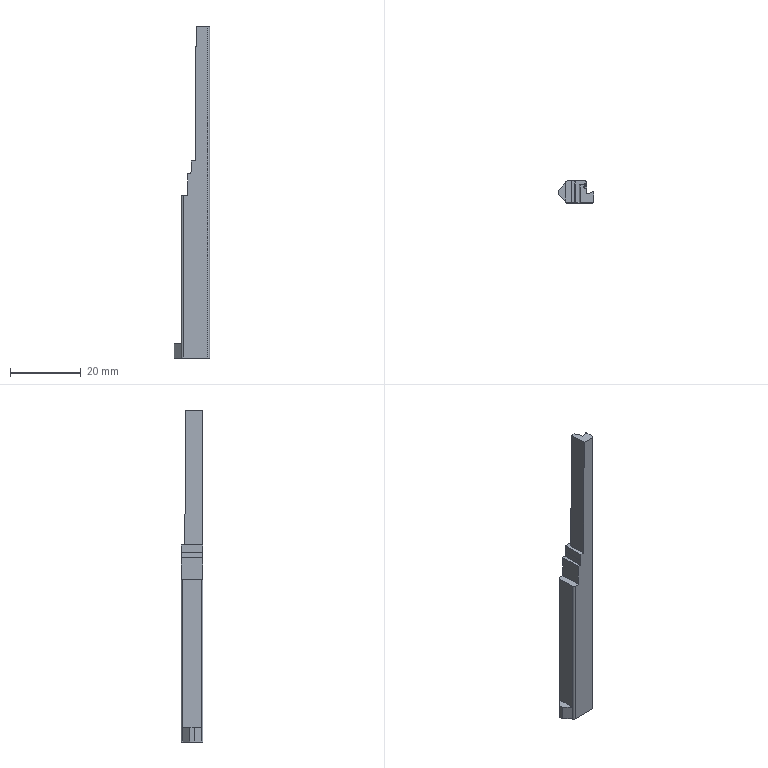Part | Creo | 1 solid | 37 faces | box 10 x 6.2 x 94.171 mm | volume 2834 mm3 | plane 23 | cylinder 8 | cone 6 | commonest cylinder face diameters 1 x4 0.6 x2 1.005 x2
STEP:
#1=CARTESIAN_POINT('',(0.,0.,0.));
#2=DIRECTION('',(0.,0.,1.));
#3=DIRECTION('',(1.,0.,0.));
#4=AXIS2_PLACEMENT_3D('',#1,#2,#3);
#5=CARTESIAN_POINT('',(-41.627,16.249,-54.09));
#6=VERTEX_POINT('',#5);
#7=CARTESIAN_POINT('',(-41.627,16.249,1.79));
#8=VERTEX_POINT('',#7);
#9=CARTESIAN_POINT('',(-41.627,16.249,-54.09));
#10=DIRECTION('',(0.,0.,1.));
#11=VECTOR('',#10,55.88);
#12=LINE('',#9,#11);
#13=EDGE_CURVE('',#6,#8,#12,.T.);
#14=ORIENTED_EDGE('',*,*,#13,.F.);
#15=CARTESIAN_POINT('',(-41.127,15.749,-54.09));
#16=VERTEX_POINT('',#15);
#17=CARTESIAN_POINT('',(-41.627,15.749,-54.09));
#18=DIRECTION('',(0.,0.,-1.));
#19=DIRECTION('',(0.,1.,0.));
#20=AXIS2_PLACEMENT_3D('',#17,#18,#19);
#21=CIRCLE('',#20,0.5);
#22=EDGE_CURVE('',#6,#16,#21,.T.);
#23=ORIENTED_EDGE('',*,*,#22,.T.);
#24=CARTESIAN_POINT('',(-41.127,15.749,1.79));
#25=VERTEX_POINT('',#24);
#26=CARTESIAN_POINT('',(-41.127,15.749,1.79));
#27=DIRECTION('',(0.,0.,-1.));
#28=VECTOR('',#27,55.88);
#29=LINE('',#26,#28);
#30=EDGE_CURVE('',#25,#16,#29,.T.);
#31=ORIENTED_EDGE('',*,*,#30,.F.);
#32=CARTESIAN_POINT('',(-41.627,15.749,1.79));
#33=DIRECTION('',(0.,0.,1.));
#34=DIRECTION('',(1.,0.,0.));
#35=AXIS2_PLACEMENT_3D('',#32,#33,#34);
#36=CIRCLE('',#35,0.5);
#37=EDGE_CURVE('',#25,#8,#36,.T.);
#38=ORIENTED_EDGE('',*,*,#37,.T.);
#39=EDGE_LOOP('',(#14,#23,#31,#38));
#40=FACE_OUTER_BOUND('',#39,.F.);
#41=CARTESIAN_POINT('',(-41.627,15.749,58.91));
#42=DIRECTION('',(0.,0.,-1.));
#43=DIRECTION('',(1.,0.,0.));
#44=AXIS2_PLACEMENT_3D('',#41,#42,#43);
#45=CYLINDRICAL_SURFACE('',#44,0.5);
#46=ADVANCED_FACE('',(#40),#45,.T.);
#47=CARTESIAN_POINT('',(-46.627,16.249,-8.027));
#48=VERTEX_POINT('',#47);
#49=CARTESIAN_POINT('',(-46.627,16.249,-54.09));
#50=VERTEX_POINT('',#49);
#51=CARTESIAN_POINT('',(-46.627,16.249,-8.027));
#52=DIRECTION('',(0.,0.,-1.));
#53=VECTOR('',#52,46.062);
#54=LINE('',#51,#53);
#55=EDGE_CURVE('',#48,#50,#54,.T.);
#56=ORIENTED_EDGE('',*,*,#55,.T.);
#57=CARTESIAN_POINT('',(-41.627,16.249,-54.09));
#58=DIRECTION('',(-1.,0.,0.));
#59=VECTOR('',#58,5.);
#60=LINE('',#57,#59);
#61=EDGE_CURVE('',#6,#50,#60,.T.);
#62=ORIENTED_EDGE('',*,*,#61,.F.);
#63=ORIENTED_EDGE('',*,*,#13,.T.);
#64=CARTESIAN_POINT('',(-44.321,16.249,1.79));
#65=VERTEX_POINT('',#64);
#66=CARTESIAN_POINT('',(-44.321,16.249,1.79));
#67=DIRECTION('',(1.,0.,0.));
#68=VECTOR('',#67,2.694);
#69=LINE('',#66,#68);
#70=EDGE_CURVE('',#65,#8,#69,.T.);
#71=ORIENTED_EDGE('',*,*,#70,.F.);
#72=CARTESIAN_POINT('',(-44.339,16.249,-0.2185));
#73=VERTEX_POINT('',#72);
#74=CARTESIAN_POINT('',(-44.321,16.249,1.79));
#75=DIRECTION('',(-0.008727,0.,-1.));
#76=VECTOR('',#75,2.009);
#77=LINE('',#74,#76);
#78=EDGE_CURVE('',#65,#73,#77,.T.);
#79=ORIENTED_EDGE('',*,*,#78,.T.);
#80=CARTESIAN_POINT('',(-44.451,16.249,-1.827));
#81=VERTEX_POINT('',#80);
#82=CARTESIAN_POINT('',(-44.451,16.249,-1.827));
#83=DIRECTION('',(0.06976,0.,0.9976));
#84=VECTOR('',#83,1.613);
#85=LINE('',#82,#84);
#86=EDGE_CURVE('',#81,#73,#85,.T.);
#87=ORIENTED_EDGE('',*,*,#86,.F.);
#88=CARTESIAN_POINT('',(-45.303,16.249,-1.827));
#89=VERTEX_POINT('',#88);
#90=CARTESIAN_POINT('',(-44.451,16.249,-1.827));
#91=DIRECTION('',(-1.,0.,0.));
#92=VECTOR('',#91,0.8522);
#93=LINE('',#90,#92);
#94=EDGE_CURVE('',#81,#89,#93,.T.);
#95=ORIENTED_EDGE('',*,*,#94,.T.);
#96=CARTESIAN_POINT('',(-45.303,16.249,-8.027));
#97=VERTEX_POINT('',#96);
#98=CARTESIAN_POINT('',(-45.303,16.249,-1.827));
#99=DIRECTION('',(0.,0.,-1.));
#100=VECTOR('',#99,6.2);
#101=LINE('',#98,#100);
#102=EDGE_CURVE('',#89,#97,#101,.T.);
#103=ORIENTED_EDGE('',*,*,#102,.T.);
#104=CARTESIAN_POINT('',(-45.303,16.249,-8.027));
#105=DIRECTION('',(-1.,0.,0.));
#106=VECTOR('',#105,1.323);
#107=LINE('',#104,#106);
#108=EDGE_CURVE('',#97,#48,#107,.T.);
#109=ORIENTED_EDGE('',*,*,#108,.T.);
#110=EDGE_LOOP('',(#56,#62,#63,#71,#79,#87,#95,#103,#109));
#111=FACE_OUTER_BOUND('',#110,.F.);
#112=CARTESIAN_POINT('',(-47.127,16.249,58.91));
#113=DIRECTION('',(0.,-1.,0.));
#114=DIRECTION('',(0.,0.,-1.));
#115=AXIS2_PLACEMENT_3D('',#112,#113,#114);
#116=PLANE('',#115);
#117=ADVANCED_FACE('',(#111),#116,.F.);
#118=CARTESIAN_POINT('',(-47.127,15.749,-8.027));
#119=VERTEX_POINT('',#118);
#120=CARTESIAN_POINT('',(-46.627,15.749,-8.027));
#121=DIRECTION('',(0.,0.,1.));
#122=DIRECTION('',(0.,1.,0.));
#123=AXIS2_PLACEMENT_3D('',#120,#121,#122);
#124=CIRCLE('',#123,0.5);
#125=EDGE_CURVE('',#48,#119,#124,.T.);
#126=ORIENTED_EDGE('',*,*,#125,.T.);
#127=CARTESIAN_POINT('',(-47.127,15.749,-50.09));
#128=VERTEX_POINT('',#127);
#129=CARTESIAN_POINT('',(-47.127,15.749,-50.09));
#130=DIRECTION('',(0.,0.,1.));
#131=VECTOR('',#130,42.062);
#132=LINE('',#129,#131);
#133=EDGE_CURVE('',#128,#119,#132,.T.);
#134=ORIENTED_EDGE('',*,*,#133,.F.);
#135=CARTESIAN_POINT('',(-47.127,15.749,-54.09));
#136=VERTEX_POINT('',#135);
#137=CARTESIAN_POINT('',(-47.127,15.749,-54.09));
#138=DIRECTION('',(0.,0.,1.));
#139=VECTOR('',#138,4.);
#140=LINE('',#137,#139);
#141=EDGE_CURVE('',#136,#128,#140,.T.);
#142=ORIENTED_EDGE('',*,*,#141,.F.);
#143=CARTESIAN_POINT('',(-46.627,15.749,-54.09));
#144=DIRECTION('',(0.,0.,-1.));
#145=DIRECTION('',(-1.,0.,0.));
#146=AXIS2_PLACEMENT_3D('',#143,#144,#145);
#147=CIRCLE('',#146,0.5);
#148=EDGE_CURVE('',#136,#50,#147,.T.);
#149=ORIENTED_EDGE('',*,*,#148,.T.);
#150=ORIENTED_EDGE('',*,*,#55,.F.);
#151=EDGE_LOOP('',(#126,#134,#142,#149,#150));
#152=FACE_OUTER_BOUND('',#151,.F.);
#153=CARTESIAN_POINT('',(-46.627,15.749,58.91));
#154=DIRECTION('',(0.,0.,-1.));
#155=DIRECTION('',(1.,0.,0.));
#156=AXIS2_PLACEMENT_3D('',#153,#154,#155);
#157=CYLINDRICAL_SURFACE('',#156,0.5);
#158=ADVANCED_FACE('',(#152),#157,.T.);
#159=ORIENTED_EDGE('',*,*,#125,.F.);
#160=ORIENTED_EDGE('',*,*,#108,.F.);
#161=CARTESIAN_POINT('',(-45.303,10.049,-8.027));
#162=VERTEX_POINT('',#161);
#163=CARTESIAN_POINT('',(-45.303,10.049,-8.027));
#164=DIRECTION('',(0.,1.,0.));
#165=VECTOR('',#164,6.2);
#166=LINE('',#163,#165);
#167=EDGE_CURVE('',#162,#97,#166,.T.);
#168=ORIENTED_EDGE('',*,*,#167,.F.);
#169=CARTESIAN_POINT('',(-46.627,10.049,-8.027));
#170=VERTEX_POINT('',#169);
#171=CARTESIAN_POINT('',(-45.303,10.049,-8.027));
#172=DIRECTION('',(-1.,0.,0.));
#173=VECTOR('',#172,1.323);
#174=LINE('',#171,#173);
#175=EDGE_CURVE('',#162,#170,#174,.T.);
#176=ORIENTED_EDGE('',*,*,#175,.T.);
#177=CARTESIAN_POINT('',(-47.127,10.549,-8.027));
#178=VERTEX_POINT('',#177);
#179=CARTESIAN_POINT('',(-46.627,10.549,-8.027));
#180=DIRECTION('',(0.,0.,1.));
#181=DIRECTION('',(-1.,0.,0.));
#182=AXIS2_PLACEMENT_3D('',#179,#180,#181);
#183=CIRCLE('',#182,0.5);
#184=EDGE_CURVE('',#178,#170,#183,.T.);
#185=ORIENTED_EDGE('',*,*,#184,.F.);
#186=CARTESIAN_POINT('',(-47.127,15.749,-8.027));
#187=DIRECTION('',(0.,-1.,0.));
#188=VECTOR('',#187,5.2);
#189=LINE('',#186,#188);
#190=EDGE_CURVE('',#119,#178,#189,.T.);
#191=ORIENTED_EDGE('',*,*,#190,.F.);
#192=EDGE_LOOP('',(#159,#160,#168,#176,#185,#191));
#193=FACE_OUTER_BOUND('',#192,.F.);
#194=CARTESIAN_POINT('',(-70.5,-0.4,-8.027));
#195=DIRECTION('',(0.,0.,-1.));
#196=DIRECTION('',(0.,-1.,0.));
#197=AXIS2_PLACEMENT_3D('',#194,#195,#196);
#198=PLANE('',#197);
#199=ADVANCED_FACE('',(#193),#198,.F.);
#200=CARTESIAN_POINT('',(-45.303,10.049,-1.827));
#201=VERTEX_POINT('',#200);
#202=CARTESIAN_POINT('',(-45.303,10.049,-1.827));
#203=DIRECTION('',(0.,0.,-1.));
#204=VECTOR('',#203,6.2);
#205=LINE('',#202,#204);
#206=EDGE_CURVE('',#201,#162,#205,.T.);
#207=ORIENTED_EDGE('',*,*,#206,.T.);
#208=ORIENTED_EDGE('',*,*,#167,.T.);
#209=ORIENTED_EDGE('',*,*,#102,.F.);
#210=CARTESIAN_POINT('',(-45.303,16.249,-1.827));
#211=DIRECTION('',(0.,-1.,0.));
#212=VECTOR('',#211,6.2);
#213=LINE('',#210,#212);
#214=EDGE_CURVE('',#89,#201,#213,.T.);
#215=ORIENTED_EDGE('',*,*,#214,.T.);
#216=EDGE_LOOP('',(#207,#208,#209,#215));
#217=FACE_OUTER_BOUND('',#216,.F.);
#218=CARTESIAN_POINT('',(-45.303,-88.35,-44.339));
#219=DIRECTION('',(-1.,0.,0.));
#220=DIRECTION('',(0.,0.,-1.));
#221=AXIS2_PLACEMENT_3D('',#218,#219,#220);
#222=PLANE('',#221);
#223=ADVANCED_FACE('',(#217),#222,.T.);
#224=ORIENTED_EDGE('',*,*,#175,.F.);
#225=ORIENTED_EDGE('',*,*,#206,.F.);
#226=CARTESIAN_POINT('',(-44.451,10.049,-1.827));
#227=VERTEX_POINT('',#226);
#228=CARTESIAN_POINT('',(-44.451,10.049,-1.827));
#229=DIRECTION('',(-1.,0.,0.));
#230=VECTOR('',#229,0.8522);
#231=LINE('',#228,#230);
#232=EDGE_CURVE('',#227,#201,#231,.T.);
#233=ORIENTED_EDGE('',*,*,#232,.F.);
#234=CARTESIAN_POINT('',(-44.339,10.049,-0.2185));
#235=VERTEX_POINT('',#234);
#236=CARTESIAN_POINT('',(-44.339,10.049,-0.2185));
#237=DIRECTION('',(-0.06976,0.,-0.9976));
#238=VECTOR('',#237,1.613);
#239=LINE('',#236,#238);
#240=EDGE_CURVE('',#235,#227,#239,.T.);
#241=ORIENTED_EDGE('',*,*,#240,.F.);
#242=CARTESIAN_POINT('',(-44.321,10.049,1.79));
#243=VERTEX_POINT('',#242);
#244=CARTESIAN_POINT('',(-44.321,10.049,1.79));
#245=DIRECTION('',(-0.008727,0.,-1.));
#246=VECTOR('',#245,2.009);
#247=LINE('',#244,#246);
#248=EDGE_CURVE('',#243,#235,#247,.T.);
#249=ORIENTED_EDGE('',*,*,#248,.F.);
#250=CARTESIAN_POINT('',(-43.276,10.049,1.79));
#251=VERTEX_POINT('',#250);
#252=CARTESIAN_POINT('',(-44.321,10.049,1.79));
#253=DIRECTION('',(1.,0.,0.));
#254=VECTOR('',#253,1.045);
#255=LINE('',#252,#254);
#256=EDGE_CURVE('',#243,#251,#255,.T.);
#257=ORIENTED_EDGE('',*,*,#256,.T.);
#258=CARTESIAN_POINT('',(-42.942,10.049,40.081));
#259=VERTEX_POINT('',#258);
#260=CARTESIAN_POINT('',(-42.942,10.049,40.081));
#261=DIRECTION('',(-0.008727,0.,-1.));
#262=VECTOR('',#261,38.292);
#263=LINE('',#260,#262);
#264=EDGE_CURVE('',#259,#251,#263,.T.);
#265=ORIENTED_EDGE('',*,*,#264,.F.);
#266=CARTESIAN_POINT('',(-39.627,10.049,40.081));
#267=VERTEX_POINT('',#266);
#268=CARTESIAN_POINT('',(-39.627,10.049,40.081));
#269=DIRECTION('',(-1.,0.,0.));
#270=VECTOR('',#269,3.315);
#271=LINE('',#268,#270);
#272=EDGE_CURVE('',#267,#259,#271,.T.);
#273=ORIENTED_EDGE('',*,*,#272,.F.);
#274=CARTESIAN_POINT('',(-39.627,10.049,-54.09));
#275=VERTEX_POINT('',#274);
#276=CARTESIAN_POINT('',(-39.627,10.049,40.081));
#277=DIRECTION('',(0.,0.,-1.));
#278=VECTOR('',#277,94.171);
#279=LINE('',#276,#278);
#280=EDGE_CURVE('',#267,#275,#279,.T.);
#281=ORIENTED_EDGE('',*,*,#280,.T.);
#282=CARTESIAN_POINT('',(-46.627,10.049,-54.09));
#283=VERTEX_POINT('',#282);
#284=CARTESIAN_POINT('',(-46.627,10.049,-54.09));
#285=DIRECTION('',(1.,0.,0.));
#286=VECTOR('',#285,7.);
#287=LINE('',#284,#286);
#288=EDGE_CURVE('',#283,#275,#287,.T.);
#289=ORIENTED_EDGE('',*,*,#288,.F.);
#290=CARTESIAN_POINT('',(-46.627,10.049,-54.09));
#291=DIRECTION('',(0.,0.,1.));
#292=VECTOR('',#291,46.062);
#293=LINE('',#290,#292);
#294=EDGE_CURVE('',#283,#170,#293,.T.);
#295=ORIENTED_EDGE('',*,*,#294,.T.);
#296=EDGE_LOOP('',(#224,#225,#233,#241,#249,#257,#265,#273,#281,#289,#295));
#297=FACE_OUTER_BOUND('',#296,.F.);
#298=CARTESIAN_POINT('',(-40.127,10.049,-45.09));
#299=DIRECTION('',(0.,-1.,0.));
#300=DIRECTION('',(0.,0.,-1.));
#301=AXIS2_PLACEMENT_3D('',#298,#299,#300);
#302=PLANE('',#301);
#303=ADVANCED_FACE('',(#297),#302,.T.);
#304=ORIENTED_EDGE('',*,*,#214,.F.);
#305=ORIENTED_EDGE('',*,*,#94,.F.);
#306=CARTESIAN_POINT('',(-44.451,10.049,-1.827));
#307=DIRECTION('',(0.,1.,0.));
#308=VECTOR('',#307,6.2);
#309=LINE('',#306,#308);
#310=EDGE_CURVE('',#227,#81,#309,.T.);
#311=ORIENTED_EDGE('',*,*,#310,.F.);
#312=ORIENTED_EDGE('',*,*,#232,.T.);
#313=EDGE_LOOP('',(#304,#305,#311,#312));
#314=FACE_OUTER_BOUND('',#313,.F.);
#315=CARTESIAN_POINT('',(-45.303,87.525,-1.827));
#316=DIRECTION('',(0.,0.,1.));
#317=DIRECTION('',(-1.,0.,0.));
#318=AXIS2_PLACEMENT_3D('',#315,#316,#317);
#319=PLANE('',#318);
#320=ADVANCED_FACE('',(#314),#319,.T.);
#321=ORIENTED_EDGE('',*,*,#310,.T.);
#322=ORIENTED_EDGE('',*,*,#86,.T.);
#323=CARTESIAN_POINT('',(-44.339,10.049,-0.2185));
#324=DIRECTION('',(0.,1.,0.));
#325=VECTOR('',#324,6.2);
#326=LINE('',#323,#325);
#327=EDGE_CURVE('',#235,#73,#326,.T.);
#328=ORIENTED_EDGE('',*,*,#327,.F.);
#329=ORIENTED_EDGE('',*,*,#240,.T.);
#330=EDGE_LOOP('',(#321,#322,#328,#329));
#331=FACE_OUTER_BOUND('',#330,.F.);
#332=CARTESIAN_POINT('',(-44.338,-87.445,-0.2167));
#333=DIRECTION('',(-0.9976,0.,0.06976));
#334=DIRECTION('',(0.,1.,0.));
#335=AXIS2_PLACEMENT_3D('',#332,#333,#334);
#336=PLANE('',#335);
#337=ADVANCED_FACE('',(#331),#336,.T.);
#338=ORIENTED_EDGE('',*,*,#327,.T.);
#339=ORIENTED_EDGE('',*,*,#78,.F.);
#340=CARTESIAN_POINT('',(-44.321,10.049,1.79));
#341=DIRECTION('',(0.,1.,0.));
#342=VECTOR('',#341,6.2);
#343=LINE('',#340,#342);
#344=EDGE_CURVE('',#243,#65,#343,.T.);
#345=ORIENTED_EDGE('',*,*,#344,.F.);
#346=ORIENTED_EDGE('',*,*,#248,.T.);
#347=EDGE_LOOP('',(#338,#339,#345,#346));
#348=FACE_OUTER_BOUND('',#347,.F.);
#349=CARTESIAN_POINT('',(-44.339,-87.445,-0.2204));
#350=DIRECTION('',(-1.,0.,0.008727));
#351=DIRECTION('',(0.,1.,0.));
#352=AXIS2_PLACEMENT_3D('',#349,#350,#351);
#353=PLANE('',#352);
#354=ADVANCED_FACE('',(#348),#353,.T.);
#355=ORIENTED_EDGE('',*,*,#256,.F.);
#356=ORIENTED_EDGE('',*,*,#344,.T.);
#357=ORIENTED_EDGE('',*,*,#70,.T.);
#358=ORIENTED_EDGE('',*,*,#37,.F.);
#359=CARTESIAN_POINT('',(-41.127,15.635,1.79));
#360=VERTEX_POINT('',#359);
#361=CARTESIAN_POINT('',(-41.127,15.749,1.79));
#362=DIRECTION('',(0.,-1.,0.));
#363=VECTOR('',#362,0.1138);
#364=LINE('',#361,#363);
#365=EDGE_CURVE('',#25,#360,#364,.T.);
#366=ORIENTED_EDGE('',*,*,#365,.T.);
#367=CARTESIAN_POINT('',(-41.283,15.657,1.79));
#368=VERTEX_POINT('',#367);
#369=CARTESIAN_POINT('',(-41.283,15.105,1.79));
#370=DIRECTION('',(0.,0.,-1.));
#371=DIRECTION('',(0.,1.,0.));
#372=AXIS2_PLACEMENT_3D('',#369,#370,#371);
#373=CIRCLE('',#372,0.5527);
#374=EDGE_CURVE('',#368,#360,#373,.T.);
#375=ORIENTED_EDGE('',*,*,#374,.F.);
#376=CARTESIAN_POINT('',(-41.283,14.552,1.79));
#377=VERTEX_POINT('',#376);
#378=CARTESIAN_POINT('',(-41.283,15.105,1.79));
#379=DIRECTION('',(0.,0.,-1.));
#380=DIRECTION('',(0.,-1.,0.));
#381=AXIS2_PLACEMENT_3D('',#378,#379,#380);
#382=CIRCLE('',#381,0.5527);
#383=EDGE_CURVE('',#377,#368,#382,.T.);
#384=ORIENTED_EDGE('',*,*,#383,.F.);
#385=CARTESIAN_POINT('',(-41.127,14.575,1.79));
#386=VERTEX_POINT('',#385);
#387=CARTESIAN_POINT('',(-41.283,15.105,1.79));
#388=DIRECTION('',(0.,0.,-1.));
#389=DIRECTION('',(0.2831,-0.9591,0.));
#390=AXIS2_PLACEMENT_3D('',#387,#388,#389);
#391=CIRCLE('',#390,0.5527);
#392=EDGE_CURVE('',#386,#377,#391,.T.);
#393=ORIENTED_EDGE('',*,*,#392,.F.);
#394=CARTESIAN_POINT('',(-41.127,14.167,1.79));
#395=VERTEX_POINT('',#394);
#396=CARTESIAN_POINT('',(-41.127,14.575,1.79));
#397=DIRECTION('',(0.,-1.,0.));
#398=VECTOR('',#397,0.4079);
#399=LINE('',#396,#398);
#400=EDGE_CURVE('',#386,#395,#399,.T.);
#401=ORIENTED_EDGE('',*,*,#400,.T.);
#402=CARTESIAN_POINT('',(-41.204,14.161,1.79));
#403=VERTEX_POINT('',#402);
#404=CARTESIAN_POINT('',(-41.127,14.167,1.79));
#405=CARTESIAN_POINT('',(-41.152,14.163,1.79));
#406=CARTESIAN_POINT('',(-41.178,14.161,1.79));
#407=CARTESIAN_POINT('',(-41.204,14.161,1.79));
#408=B_SPLINE_CURVE_WITH_KNOTS('',3,(#404,#405,#406,#407),.UNSPECIFIED.,.F.,.F.,(4,4),(0.,1.),.UNSPECIFIED.);
#409=EDGE_CURVE('',#395,#403,#408,.T.);
#410=ORIENTED_EDGE('',*,*,#409,.T.);
#411=CARTESIAN_POINT('',(-41.363,14.161,1.79));
#412=VERTEX_POINT('',#411);
#413=CARTESIAN_POINT('',(-41.204,14.161,1.79));
#414=DIRECTION('',(-1.,0.,-0.000000005));
#415=VECTOR('',#414,0.1592);
#416=LINE('',#413,#415);
#417=EDGE_CURVE('',#403,#412,#416,.T.);
#418=ORIENTED_EDGE('',*,*,#417,.T.);
#419=CARTESIAN_POINT('',(-41.865,14.663,1.79));
#420=VERTEX_POINT('',#419);
#421=CARTESIAN_POINT('',(-41.363,14.161,1.79));
#422=CARTESIAN_POINT('',(-41.53,14.161,1.79));
#423=CARTESIAN_POINT('',(-41.739,14.288,1.79));
#424=CARTESIAN_POINT('',(-41.865,14.496,1.79));
#425=CARTESIAN_POINT('',(-41.865,14.663,1.79));
#426=B_SPLINE_CURVE_WITH_KNOTS('',3,(#421,#422,#423,#424,#425),.UNSPECIFIED.,.F.,.F.,(4,1,4),(0.,0.5,1.),.UNSPECIFIED.);
#427=EDGE_CURVE('',#412,#420,#426,.T.);
#428=ORIENTED_EDGE('',*,*,#427,.T.);
#429=CARTESIAN_POINT('',(-41.865,15.153,1.79));
#430=VERTEX_POINT('',#429);
#431=CARTESIAN_POINT('',(-41.865,14.663,1.79));
#432=DIRECTION('',(0.,1.,0.));
#433=VECTOR('',#432,0.49);
#434=LINE('',#431,#433);
#435=EDGE_CURVE('',#420,#430,#434,.T.);
#436=ORIENTED_EDGE('',*,*,#435,.T.);
#437=CARTESIAN_POINT('',(-43.276,15.166,1.79));
#438=VERTEX_POINT('',#437);
#439=CARTESIAN_POINT('',(-41.865,15.153,1.79));
#440=DIRECTION('',(-1.,0.008727,0.));
#441=VECTOR('',#440,1.41);
#442=LINE('',#439,#441);
#443=EDGE_CURVE('',#430,#438,#442,.T.);
#444=ORIENTED_EDGE('',*,*,#443,.T.);
#445=CARTESIAN_POINT('',(-43.276,10.049,1.79));
#446=DIRECTION('',(0.,1.,0.));
#447=VECTOR('',#446,5.117);
#448=LINE('',#445,#447);
#449=EDGE_CURVE('',#251,#438,#448,.T.);
#450=ORIENTED_EDGE('',*,*,#449,.F.);
#451=EDGE_LOOP('',(#355,#356,#357,#358,#366,#375,#384,#393,#401,#410,#418,#428,#436,#444,#450));
#452=FACE_OUTER_BOUND('',#451,.F.);
#453=CARTESIAN_POINT('',(-0.07825,87.525,1.79));
#454=DIRECTION('',(0.,0.,-1.));
#455=DIRECTION('',(0.,-1.,0.));
#456=AXIS2_PLACEMENT_3D('',#453,#454,#455);
#457=PLANE('',#456);
#458=ADVANCED_FACE('',(#452),#457,.F.);
#459=CARTESIAN_POINT('',(-41.127,14.084,23.814));
#460=VERTEX_POINT('',#459);
#461=CARTESIAN_POINT('',(-41.127,14.027,40.081));
#462=VERTEX_POINT('',#461);
#463=CARTESIAN_POINT('',(-41.127,14.084,23.814));
#464=DIRECTION('',(0.,-0.003491,1.));
#465=VECTOR('',#464,16.267);
#466=LINE('',#463,#465);
#467=EDGE_CURVE('',#460,#462,#466,.T.);
#468=ORIENTED_EDGE('',*,*,#467,.F.);
#469=CARTESIAN_POINT('',(-41.127,14.167,1.79));
#470=CARTESIAN_POINT('',(-41.127,14.137,9.132));
#471=CARTESIAN_POINT('',(-41.127,14.11,16.473));
#472=CARTESIAN_POINT('',(-41.127,14.084,23.814));
#473=B_SPLINE_CURVE_WITH_KNOTS('',3,(#469,#470,#471,#472),.UNSPECIFIED.,.F.,.F.,(4,4),(0.,1.),.UNSPECIFIED.);
#474=EDGE_CURVE('',#395,#460,#473,.T.);
#475=ORIENTED_EDGE('',*,*,#474,.F.);
#476=ORIENTED_EDGE('',*,*,#400,.F.);
#477=CARTESIAN_POINT('',(-41.127,14.584,0.7855));
#478=VERTEX_POINT('',#477);
#479=CARTESIAN_POINT('',(-41.127,14.584,0.7855));
#480=CARTESIAN_POINT('',(-41.127,14.581,1.12));
#481=CARTESIAN_POINT('',(-41.127,14.578,1.455));
#482=B_SPLINE_CURVE_WITH_KNOTS('',3,(#479,#480,#481,#385),.UNSPECIFIED.,.F.,.F.,(4,4),(0.,1.),.UNSPECIFIED.);
#483=EDGE_CURVE('',#478,#386,#482,.T.);
#484=ORIENTED_EDGE('',*,*,#483,.F.);
#485=CARTESIAN_POINT('',(-41.127,14.923,0.484));
#486=VERTEX_POINT('',#485);
#487=CARTESIAN_POINT('',(-41.127,14.923,0.484));
#488=CARTESIAN_POINT('',(-41.127,14.884,0.5131));
#489=CARTESIAN_POINT('',(-41.127,14.808,0.5754));
#490=CARTESIAN_POINT('',(-41.127,14.696,0.6777));
#491=CARTESIAN_POINT('',(-41.127,14.622,0.7494));
#492=B_SPLINE_CURVE_WITH_KNOTS('',3,(#487,#488,#489,#490,#491,#477),.UNSPECIFIED.,.F.,.F.,(4,1,1,4),(0.,0.3333,0.6667,1.),.UNSPECIFIED.);
#493=EDGE_CURVE('',#486,#478,#492,.T.);
#494=ORIENTED_EDGE('',*,*,#493,.F.);
#495=CARTESIAN_POINT('',(-41.127,15.286,0.484));
#496=VERTEX_POINT('',#495);
#497=CARTESIAN_POINT('',(-41.127,15.286,0.484));
#498=DIRECTION('',(0.,-1.,0.));
#499=VECTOR('',#498,0.3635);
#500=LINE('',#497,#499);
#501=EDGE_CURVE('',#496,#486,#500,.T.);
#502=ORIENTED_EDGE('',*,*,#501,.F.);
#503=CARTESIAN_POINT('',(-41.127,15.626,0.7855));
#504=VERTEX_POINT('',#503);
#505=CARTESIAN_POINT('',(-41.127,15.626,0.7855));
#506=CARTESIAN_POINT('',(-41.127,15.588,0.7494));
#507=CARTESIAN_POINT('',(-41.127,15.513,0.6782));
#508=CARTESIAN_POINT('',(-41.127,15.401,0.5755));
#509=CARTESIAN_POINT('',(-41.127,15.325,0.5131));
#510=B_SPLINE_CURVE_WITH_KNOTS('',3,(#505,#506,#507,#508,#509,#495),.UNSPECIFIED.,.F.,.F.,(4,1,1,4),(0.,0.3333,0.6667,1.),.UNSPECIFIED.);
#511=EDGE_CURVE('',#504,#496,#510,.T.);
#512=ORIENTED_EDGE('',*,*,#511,.F.);
#513=CARTESIAN_POINT('',(-41.127,15.635,1.79));
#514=CARTESIAN_POINT('',(-41.127,15.632,1.455));
#515=CARTESIAN_POINT('',(-41.127,15.629,1.12));
#516=B_SPLINE_CURVE_WITH_KNOTS('',3,(#513,#514,#515,#503),.UNSPECIFIED.,.F.,.F.,(4,4),(0.,1.),.UNSPECIFIED.);
#517=EDGE_CURVE('',#360,#504,#516,.T.);
#518=ORIENTED_EDGE('',*,*,#517,.F.);
#519=ORIENTED_EDGE('',*,*,#365,.F.);
#520=ORIENTED_EDGE('',*,*,#30,.T.);
#521=CARTESIAN_POINT('',(-41.127,12.823,-54.09));
#522=VERTEX_POINT('',#521);
#523=CARTESIAN_POINT('',(-41.127,12.823,-54.09));
#524=DIRECTION('',(0.,1.,0.));
#525=VECTOR('',#524,2.926);
#526=LINE('',#523,#525);
#527=EDGE_CURVE('',#522,#16,#526,.T.);
#528=ORIENTED_EDGE('',*,*,#527,.F.);
#529=CARTESIAN_POINT('',(-41.127,12.823,40.081));
#530=VERTEX_POINT('',#529);
#531=CARTESIAN_POINT('',(-41.127,12.823,-54.09));
#532=DIRECTION('',(0.,0.,1.));
#533=VECTOR('',#532,94.171);
#534=LINE('',#531,#533);
#535=EDGE_CURVE('',#522,#530,#534,.T.);
#536=ORIENTED_EDGE('',*,*,#535,.T.);
#537=CARTESIAN_POINT('',(-41.127,12.823,40.081));
#538=DIRECTION('',(0.,1.,0.));
#539=VECTOR('',#538,1.204);
#540=LINE('',#537,#539);
#541=EDGE_CURVE('',#530,#462,#540,.T.);
#542=ORIENTED_EDGE('',*,*,#541,.T.);
#543=EDGE_LOOP('',(#468,#475,#476,#484,#494,#502,#512,#518,#519,#520,#528,#536,#542));
#544=FACE_OUTER_BOUND('',#543,.F.);
#545=CARTESIAN_POINT('',(-41.127,16.249,58.91));
#546=DIRECTION('',(-1.,0.,0.));
#547=DIRECTION('',(0.,0.,-1.));
#548=AXIS2_PLACEMENT_3D('',#545,#546,#547);
#549=PLANE('',#548);
#550=ADVANCED_FACE('',(#544),#549,.F.);
#551=CARTESIAN_POINT('',(-41.497,14.027,40.081));
#552=VERTEX_POINT('',#551);
#553=CARTESIAN_POINT('',(-41.127,14.027,40.081));
#554=DIRECTION('',(-1.,0.,-0.000000002));
#555=VECTOR('',#554,0.3698);
#556=LINE('',#553,#555);
#557=EDGE_CURVE('',#462,#552,#556,.T.);
#558=ORIENTED_EDGE('',*,*,#557,.T.);
#559=CARTESIAN_POINT('',(-41.363,14.161,1.79));
#560=DIRECTION('',(-0.003491,-0.003491,1.));
#561=VECTOR('',#560,38.291);
#562=LINE('',#559,#561);
#563=EDGE_CURVE('',#412,#552,#562,.T.);
#564=ORIENTED_EDGE('',*,*,#563,.F.);
#565=ORIENTED_EDGE('',*,*,#417,.F.);
#566=CARTESIAN_POINT('',(-41.127,14.084,23.814));
#567=DIRECTION('',(-0.003491,0.003491,-1.));
#568=VECTOR('',#567,22.024);
#569=LINE('',#566,#568);
#570=EDGE_CURVE('',#460,#403,#569,.T.);
#571=ORIENTED_EDGE('',*,*,#570,.F.);
#572=ORIENTED_EDGE('',*,*,#467,.T.);
#573=EDGE_LOOP('',(#558,#564,#565,#571,#572));
#574=FACE_OUTER_BOUND('',#573,.F.);
#575=CARTESIAN_POINT('',(-37.97,14.039,36.563));
#576=DIRECTION('',(0.,-1.,-0.003491));
#577=DIRECTION('',(1.,0.,0.));
#578=AXIS2_PLACEMENT_3D('',#575,#576,#577);
#579=PLANE('',#578);
#580=ADVANCED_FACE('',(#574),#579,.F.);
#581=ORIENTED_EDGE('',*,*,#541,.F.);
#582=CARTESIAN_POINT('',(-40.7,12.551,40.081));
#583=VERTEX_POINT('',#582);
#584=CARTESIAN_POINT('',(-40.827,12.823,40.081));
#585=DIRECTION('',(0.,0.,-1.));
#586=DIRECTION('',(0.4226,-0.9063,0.));
#587=AXIS2_PLACEMENT_3D('',#584,#585,#586);
#588=CIRCLE('',#587,0.3);
#589=EDGE_CURVE('',#583,#530,#588,.T.);
#590=ORIENTED_EDGE('',*,*,#589,.F.);
#591=CARTESIAN_POINT('',(-39.554,13.086,40.081));
#592=VERTEX_POINT('',#591);
#593=CARTESIAN_POINT('',(-39.554,13.086,40.081));
#594=DIRECTION('',(-0.9063,-0.4226,0.));
#595=VECTOR('',#594,1.265);
#596=LINE('',#593,#595);
#597=EDGE_CURVE('',#592,#583,#596,.T.);
#598=ORIENTED_EDGE('',*,*,#597,.F.);
#599=CARTESIAN_POINT('',(-39.127,12.814,40.081));
#600=VERTEX_POINT('',#599);
#601=CARTESIAN_POINT('',(-39.427,12.814,40.081));
#602=DIRECTION('',(0.,0.,1.));
#603=DIRECTION('',(1.,0.,0.));
#604=AXIS2_PLACEMENT_3D('',#601,#602,#603);
#605=CIRCLE('',#604,0.3);
#606=EDGE_CURVE('',#600,#592,#605,.T.);
#607=ORIENTED_EDGE('',*,*,#606,.F.);
#608=CARTESIAN_POINT('',(-39.127,10.549,40.081));
#609=VERTEX_POINT('',#608);
#610=CARTESIAN_POINT('',(-39.127,12.814,40.081));
#611=DIRECTION('',(0.,-1.,0.));
#612=VECTOR('',#611,2.265);
#613=LINE('',#610,#612);
#614=EDGE_CURVE('',#600,#609,#613,.T.);
#615=ORIENTED_EDGE('',*,*,#614,.T.);
#616=CARTESIAN_POINT('',(-39.627,10.549,40.081));
#617=DIRECTION('',(0.,0.,1.));
#618=DIRECTION('',(0.,-1.,0.));
#619=AXIS2_PLACEMENT_3D('',#616,#617,#618);
#620=CIRCLE('',#619,0.5);
#621=EDGE_CURVE('',#267,#609,#620,.T.);
#622=ORIENTED_EDGE('',*,*,#621,.F.);
#623=ORIENTED_EDGE('',*,*,#272,.T.);
#624=CARTESIAN_POINT('',(-42.942,15.029,40.081));
#625=VERTEX_POINT('',#624);
#626=CARTESIAN_POINT('',(-42.942,10.049,40.081));
#627=DIRECTION('',(0.,1.,0.));
#628=VECTOR('',#627,4.98);
#629=LINE('',#626,#628);
#630=EDGE_CURVE('',#259,#625,#629,.T.);
#631=ORIENTED_EDGE('',*,*,#630,.T.);
#632=CARTESIAN_POINT('',(-41.999,15.021,40.081));
#633=VERTEX_POINT('',#632);
#634=CARTESIAN_POINT('',(-42.942,15.029,40.081));
#635=DIRECTION('',(1.,-0.008727,0.));
#636=VECTOR('',#635,0.9426);
#637=LINE('',#634,#636);
#638=EDGE_CURVE('',#625,#633,#637,.T.);
#639=ORIENTED_EDGE('',*,*,#638,.T.);
#640=CARTESIAN_POINT('',(-41.999,14.53,40.081));
#641=VERTEX_POINT('',#640);
#642=CARTESIAN_POINT('',(-41.999,14.53,40.081));
#643=DIRECTION('',(0.,1.,0.000000002));
#644=VECTOR('',#643,0.4912);
#645=LINE('',#642,#644);
#646=EDGE_CURVE('',#641,#633,#645,.T.);
#647=ORIENTED_EDGE('',*,*,#646,.F.);
#648=CARTESIAN_POINT('',(-41.999,14.53,40.081));
#649=CARTESIAN_POINT('',(-41.999,14.362,40.081));
#650=CARTESIAN_POINT('',(-41.872,14.154,40.081));
#651=CARTESIAN_POINT('',(-41.664,14.027,40.081));
#652=B_SPLINE_CURVE_WITH_KNOTS('',3,(#648,#649,#650,#651,#551),.UNSPECIFIED.,.F.,.F.,(4,1,4),(0.,0.5,1.),.UNSPECIFIED.);
#653=EDGE_CURVE('',#641,#552,#652,.T.);
#654=ORIENTED_EDGE('',*,*,#653,.T.);
#655=ORIENTED_EDGE('',*,*,#557,.F.);
#656=EDGE_LOOP('',(#581,#590,#598,#607,#615,#622,#623,#631,#639,#647,#654,#655));
#657=FACE_OUTER_BOUND('',#656,.F.);
#658=CARTESIAN_POINT('',(-17.817,-88.35,40.081));
#659=DIRECTION('',(0.,0.,1.));
#660=DIRECTION('',(-1.,0.,0.));
#661=AXIS2_PLACEMENT_3D('',#658,#659,#660);
#662=PLANE('',#661);
#663=ADVANCED_FACE('',(#657),#662,.T.);
#664=ORIENTED_EDGE('',*,*,#535,.F.);
#665=CARTESIAN_POINT('',(-40.7,12.551,-54.09));
#666=VERTEX_POINT('',#665);
#667=CARTESIAN_POINT('',(-40.827,12.823,-54.09));
#668=DIRECTION('',(0.,0.,1.));
#669=DIRECTION('',(-1.,0.,0.));
#670=AXIS2_PLACEMENT_3D('',#667,#668,#669);
#671=CIRCLE('',#670,0.3);
#672=EDGE_CURVE('',#522,#666,#671,.T.);
#673=ORIENTED_EDGE('',*,*,#672,.T.);
#674=CARTESIAN_POINT('',(-40.7,12.551,40.081));
#675=DIRECTION('',(0.,0.,-1.));
#676=VECTOR('',#675,94.171);
#677=LINE('',#674,#676);
#678=EDGE_CURVE('',#583,#666,#677,.T.);
#679=ORIENTED_EDGE('',*,*,#678,.F.);
#680=ORIENTED_EDGE('',*,*,#589,.T.);
#681=EDGE_LOOP('',(#664,#673,#679,#680));
#682=FACE_OUTER_BOUND('',#681,.F.);
#683=CARTESIAN_POINT('',(-40.827,12.823,58.91));
#684=DIRECTION('',(0.,0.,-1.));
#685=DIRECTION('',(1.,0.,0.));
#686=AXIS2_PLACEMENT_3D('',#683,#684,#685);
#687=CYLINDRICAL_SURFACE('',#686,0.3);
#688=ADVANCED_FACE('',(#682),#687,.F.);
#689=CARTESIAN_POINT('',(-49.127,12.549,-54.09));
#690=VERTEX_POINT('',#689);
#691=CARTESIAN_POINT('',(-49.127,13.749,-54.09));
#692=VERTEX_POINT('',#691);
#693=CARTESIAN_POINT('',(-49.127,12.549,-54.09));
#694=DIRECTION('',(0.,1.,0.));
#695=VECTOR('',#694,1.2);
#696=LINE('',#693,#695);
#697=EDGE_CURVE('',#690,#692,#696,.T.);
#698=ORIENTED_EDGE('',*,*,#697,.F.);
#699=CARTESIAN_POINT('',(-47.127,10.549,-54.09));
#700=VERTEX_POINT('',#699);
#701=CARTESIAN_POINT('',(-47.127,10.549,-54.09));
#702=DIRECTION('',(-0.7071,0.7071,0.));
#703=VECTOR('',#702,2.828);
#704=LINE('',#701,#703);
#705=EDGE_CURVE('',#700,#690,#704,.T.);
#706=ORIENTED_EDGE('',*,*,#705,.F.);
#707=CARTESIAN_POINT('',(-46.627,10.549,-54.09));
#708=DIRECTION('',(0.,0.,-1.));
#709=DIRECTION('',(0.,-1.,0.));
#710=AXIS2_PLACEMENT_3D('',#707,#708,#709);
#711=CIRCLE('',#710,0.5);
#712=EDGE_CURVE('',#283,#700,#711,.T.);
#713=ORIENTED_EDGE('',*,*,#712,.F.);
#714=ORIENTED_EDGE('',*,*,#288,.T.);
#715=CARTESIAN_POINT('',(-39.127,10.549,-54.09));
#716=VERTEX_POINT('',#715);
#717=CARTESIAN_POINT('',(-39.627,10.549,-54.09));
#718=DIRECTION('',(0.,0.,-1.));
#719=DIRECTION('',(1.,0.,0.));
#720=AXIS2_PLACEMENT_3D('',#717,#718,#719);
#721=CIRCLE('',#720,0.5);
#722=EDGE_CURVE('',#716,#275,#721,.T.);
#723=ORIENTED_EDGE('',*,*,#722,.F.);
#724=CARTESIAN_POINT('',(-39.127,12.814,-54.09));
#725=VERTEX_POINT('',#724);
#726=CARTESIAN_POINT('',(-39.127,10.549,-54.09));
#727=DIRECTION('',(0.,1.,0.));
#728=VECTOR('',#727,2.265);
#729=LINE('',#726,#728);
#730=EDGE_CURVE('',#716,#725,#729,.T.);
#731=ORIENTED_EDGE('',*,*,#730,.T.);
#732=CARTESIAN_POINT('',(-39.554,13.086,-54.09));
#733=VERTEX_POINT('',#732);
#734=CARTESIAN_POINT('',(-39.427,12.814,-54.09));
#735=DIRECTION('',(0.,0.,-1.));
#736=DIRECTION('',(-0.4226,0.9063,0.));
#737=AXIS2_PLACEMENT_3D('',#734,#735,#736);
#738=CIRCLE('',#737,0.3);
#739=EDGE_CURVE('',#733,#725,#738,.T.);
#740=ORIENTED_EDGE('',*,*,#739,.F.);
#741=CARTESIAN_POINT('',(-40.7,12.551,-54.09));
#742=DIRECTION('',(0.9063,0.4226,0.));
#743=VECTOR('',#742,1.265);
#744=LINE('',#741,#743);
#745=EDGE_CURVE('',#666,#733,#744,.T.);
#746=ORIENTED_EDGE('',*,*,#745,.F.);
#747=ORIENTED_EDGE('',*,*,#672,.F.);
#748=ORIENTED_EDGE('',*,*,#527,.T.);
#749=ORIENTED_EDGE('',*,*,#22,.F.);
#750=ORIENTED_EDGE('',*,*,#61,.T.);
#751=ORIENTED_EDGE('',*,*,#148,.F.);
#752=CARTESIAN_POINT('',(-49.127,13.749,-54.09));
#753=DIRECTION('',(0.7071,0.7071,0.));
#754=VECTOR('',#753,2.828);
#755=LINE('',#752,#754);
#756=EDGE_CURVE('',#692,#136,#755,.T.);
#757=ORIENTED_EDGE('',*,*,#756,.F.);
#758=EDGE_LOOP('',(#698,#706,#713,#714,#723,#731,#740,#746,#747,#748,#749,#750,#751,#757));
#759=FACE_OUTER_BOUND('',#758,.F.);
#760=CARTESIAN_POINT('',(0.,0.,-54.09));
#761=DIRECTION('',(0.,0.,-1.));
#762=DIRECTION('',(-1.,0.,0.));
#763=AXIS2_PLACEMENT_3D('',#760,#761,#762);
#764=PLANE('',#763);
#765=ADVANCED_FACE('',(#759),#764,.T.);
#766=CARTESIAN_POINT('',(-49.127,13.749,-50.09));
#767=VERTEX_POINT('',#766);
#768=CARTESIAN_POINT('',(-49.127,12.549,-50.09));
#769=VERTEX_POINT('',#768);
#770=CARTESIAN_POINT('',(-49.127,13.749,-50.09));
#771=DIRECTION('',(0.,-1.,0.));
#772=VECTOR('',#771,1.2);
#773=LINE('',#770,#772);
#774=EDGE_CURVE('',#767,#769,#773,.T.);
#775=ORIENTED_EDGE('',*,*,#774,.T.);
#776=CARTESIAN_POINT('',(-49.127,12.549,-50.09));
#777=DIRECTION('',(0.,0.,-1.));
#778=VECTOR('',#777,4.);
#779=LINE('',#776,#778);
#780=EDGE_CURVE('',#769,#690,#779,.T.);
#781=ORIENTED_EDGE('',*,*,#780,.T.);
#782=ORIENTED_EDGE('',*,*,#697,.T.);
#783=CARTESIAN_POINT('',(-49.127,13.749,-54.09));
#784=DIRECTION('',(0.,0.,1.));
#785=VECTOR('',#784,4.);
#786=LINE('',#783,#785);
#787=EDGE_CURVE('',#692,#767,#786,.T.);
#788=ORIENTED_EDGE('',*,*,#787,.T.);
#789=EDGE_LOOP('',(#775,#781,#782,#788));
#790=FACE_OUTER_BOUND('',#789,.F.);
#791=CARTESIAN_POINT('',(-49.127,13.149,-54.09));
#792=DIRECTION('',(-1.,0.,0.));
#793=DIRECTION('',(0.,0.,1.));
#794=AXIS2_PLACEMENT_3D('',#791,#792,#793);
#795=PLANE('',#794);
#796=ADVANCED_FACE('',(#790),#795,.T.);
#797=CARTESIAN_POINT('',(-47.127,10.549,-50.09));
#798=VERTEX_POINT('',#797);
#799=CARTESIAN_POINT('',(-47.127,10.549,-50.09));
#800=DIRECTION('',(0.,1.,0.));
#801=VECTOR('',#800,5.2);
#802=LINE('',#799,#801);
#803=EDGE_CURVE('',#798,#128,#802,.T.);
#804=ORIENTED_EDGE('',*,*,#803,.F.);
#805=CARTESIAN_POINT('',(-49.127,12.549,-50.09));
#806=DIRECTION('',(0.7071,-0.7071,0.));
#807=VECTOR('',#806,2.828);
#808=LINE('',#805,#807);
#809=EDGE_CURVE('',#769,#798,#808,.T.);
#810=ORIENTED_EDGE('',*,*,#809,.F.);
#811=ORIENTED_EDGE('',*,*,#774,.F.);
#812=CARTESIAN_POINT('',(-47.127,15.749,-50.09));
#813=DIRECTION('',(-0.7071,-0.7071,0.));
#814=VECTOR('',#813,2.828);
#815=LINE('',#812,#814);
#816=EDGE_CURVE('',#128,#767,#815,.T.);
#817=ORIENTED_EDGE('',*,*,#816,.F.);
#818=EDGE_LOOP('',(#804,#810,#811,#817));
#819=FACE_OUTER_BOUND('',#818,.F.);
#820=CARTESIAN_POINT('',(-47.627,13.149,-50.09));
#821=DIRECTION('',(0.,0.,1.));
#822=DIRECTION('',(1.,0.,0.));
#823=AXIS2_PLACEMENT_3D('',#820,#821,#822);
#824=PLANE('',#823);
#825=ADVANCED_FACE('',(#819),#824,.T.);
#826=CARTESIAN_POINT('',(-47.127,10.549,-8.027));
#827=DIRECTION('',(0.,0.,-1.));
#828=VECTOR('',#827,42.062);
#829=LINE('',#826,#828);
#830=EDGE_CURVE('',#178,#798,#829,.T.);
#831=ORIENTED_EDGE('',*,*,#830,.T.);
#832=ORIENTED_EDGE('',*,*,#803,.T.);
#833=ORIENTED_EDGE('',*,*,#133,.T.);
#834=ORIENTED_EDGE('',*,*,#190,.T.);
#835=EDGE_LOOP('',(#831,#832,#833,#834));
#836=FACE_OUTER_BOUND('',#835,.F.);
#837=CARTESIAN_POINT('',(-47.127,11.249,58.91));
#838=DIRECTION('',(1.,0.,0.));
#839=DIRECTION('',(0.,0.,1.));
#840=AXIS2_PLACEMENT_3D('',#837,#838,#839);
#841=PLANE('',#840);
#842=ADVANCED_FACE('',(#836),#841,.F.);
#843=ORIENTED_EDGE('',*,*,#184,.T.);
#844=ORIENTED_EDGE('',*,*,#294,.F.);
#845=ORIENTED_EDGE('',*,*,#712,.T.);
#846=CARTESIAN_POINT('',(-47.127,10.549,-50.09));
#847=DIRECTION('',(0.,0.,-1.));
#848=VECTOR('',#847,4.);
#849=LINE('',#846,#848);
#850=EDGE_CURVE('',#798,#700,#849,.T.);
#851=ORIENTED_EDGE('',*,*,#850,.F.);
#852=ORIENTED_EDGE('',*,*,#830,.F.);
#853=EDGE_LOOP('',(#843,#844,#845,#851,#852));
#854=FACE_OUTER_BOUND('',#853,.F.);
#855=CARTESIAN_POINT('',(-46.627,10.549,58.91));
#856=DIRECTION('',(0.,0.,1.));
#857=DIRECTION('',(-1.,0.,0.));
#858=AXIS2_PLACEMENT_3D('',#855,#856,#857);
#859=CYLINDRICAL_SURFACE('',#858,0.5);
#860=ADVANCED_FACE('',(#854),#859,.T.);
#861=ORIENTED_EDGE('',*,*,#705,.T.);
#862=ORIENTED_EDGE('',*,*,#780,.F.);
#863=ORIENTED_EDGE('',*,*,#809,.T.);
#864=ORIENTED_EDGE('',*,*,#850,.T.);
#865=EDGE_LOOP('',(#861,#862,#863,#864));
#866=FACE_OUTER_BOUND('',#865,.F.);
#867=CARTESIAN_POINT('',(-49.127,12.549,-54.09));
#868=DIRECTION('',(0.7071,0.7071,0.));
#869=DIRECTION('',(0.,0.,1.));
#870=AXIS2_PLACEMENT_3D('',#867,#868,#869);
#871=PLANE('',#870);
#872=ADVANCED_FACE('',(#866),#871,.F.);
#873=ORIENTED_EDGE('',*,*,#756,.T.);
#874=ORIENTED_EDGE('',*,*,#141,.T.);
#875=ORIENTED_EDGE('',*,*,#816,.T.);
#876=ORIENTED_EDGE('',*,*,#787,.F.);
#877=EDGE_LOOP('',(#873,#874,#875,#876));
#878=FACE_OUTER_BOUND('',#877,.F.);
#879=CARTESIAN_POINT('',(-47.127,15.749,-54.09));
#880=DIRECTION('',(0.7071,-0.7071,0.));
#881=DIRECTION('',(0.,0.,1.));
#882=AXIS2_PLACEMENT_3D('',#879,#880,#881);
#883=PLANE('',#882);
#884=ADVANCED_FACE('',(#878),#883,.F.);
#885=ORIENTED_EDGE('',*,*,#722,.T.);
#886=ORIENTED_EDGE('',*,*,#280,.F.);
#887=ORIENTED_EDGE('',*,*,#621,.T.);
#888=CARTESIAN_POINT('',(-39.127,10.549,-54.09));
#889=DIRECTION('',(0.,0.,1.));
#890=VECTOR('',#889,94.171);
#891=LINE('',#888,#890);
#892=EDGE_CURVE('',#716,#609,#891,.T.);
#893=ORIENTED_EDGE('',*,*,#892,.F.);
#894=EDGE_LOOP('',(#885,#886,#887,#893));
#895=FACE_OUTER_BOUND('',#894,.F.);
#896=CARTESIAN_POINT('',(-39.627,10.549,-45.09));
#897=DIRECTION('',(0.,0.,1.));
#898=DIRECTION('',(-1.,0.,0.));
#899=AXIS2_PLACEMENT_3D('',#896,#897,#898);
#900=CYLINDRICAL_SURFACE('',#899,0.5);
#901=ADVANCED_FACE('',(#895),#900,.T.);
#902=ORIENTED_EDGE('',*,*,#730,.F.);
#903=ORIENTED_EDGE('',*,*,#892,.T.);
#904=ORIENTED_EDGE('',*,*,#614,.F.);
#905=CARTESIAN_POINT('',(-39.127,12.814,40.081));
#906=DIRECTION('',(0.,0.,-1.));
#907=VECTOR('',#906,94.171);
#908=LINE('',#905,#907);
#909=EDGE_CURVE('',#600,#725,#908,.T.);
#910=ORIENTED_EDGE('',*,*,#909,.T.);
#911=EDGE_LOOP('',(#902,#903,#904,#910));
#912=FACE_OUTER_BOUND('',#911,.F.);
#913=CARTESIAN_POINT('',(-39.127,11.499,-45.09));
#914=DIRECTION('',(1.,0.,0.));
#915=DIRECTION('',(0.,0.,1.));
#916=AXIS2_PLACEMENT_3D('',#913,#914,#915);
#917=PLANE('',#916);
#918=ADVANCED_FACE('',(#912),#917,.T.);
#919=ORIENTED_EDGE('',*,*,#739,.T.);
#920=ORIENTED_EDGE('',*,*,#909,.F.);
#921=ORIENTED_EDGE('',*,*,#606,.T.);
#922=CARTESIAN_POINT('',(-39.554,13.086,-54.09));
#923=DIRECTION('',(0.,0.,1.));
#924=VECTOR('',#923,94.171);
#925=LINE('',#922,#924);
#926=EDGE_CURVE('',#733,#592,#925,.T.);
#927=ORIENTED_EDGE('',*,*,#926,.F.);
#928=EDGE_LOOP('',(#919,#920,#921,#927));
#929=FACE_OUTER_BOUND('',#928,.F.);
#930=CARTESIAN_POINT('',(-39.427,12.814,-45.09));
#931=DIRECTION('',(0.,0.,-1.));
#932=DIRECTION('',(1.,0.,0.));
#933=AXIS2_PLACEMENT_3D('',#930,#931,#932);
#934=CYLINDRICAL_SURFACE('',#933,0.3);
#935=ADVANCED_FACE('',(#929),#934,.T.);
#936=ORIENTED_EDGE('',*,*,#745,.T.);
#937=ORIENTED_EDGE('',*,*,#926,.T.);
#938=ORIENTED_EDGE('',*,*,#597,.T.);
#939=ORIENTED_EDGE('',*,*,#678,.T.);
#940=EDGE_LOOP('',(#936,#937,#938,#939));
#941=FACE_OUTER_BOUND('',#940,.F.);
#942=CARTESIAN_POINT('',(-39.127,13.285,-45.09));
#943=DIRECTION('',(0.4226,-0.9063,0.));
#944=DIRECTION('',(-0.9063,-0.4226,0.));
#945=AXIS2_PLACEMENT_3D('',#942,#943,#944);
#946=PLANE('',#945);
#947=ADVANCED_FACE('',(#941),#946,.F.);
#948=ORIENTED_EDGE('',*,*,#449,.T.);
#949=CARTESIAN_POINT('',(-42.943,15.029,39.962));
#950=VERTEX_POINT('',#949);
#951=CARTESIAN_POINT('',(-42.943,15.029,39.962));
#952=DIRECTION('',(-0.008726,0.003567,-1.));
#953=VECTOR('',#952,38.174);
#954=LINE('',#951,#953);
#955=EDGE_CURVE('',#950,#438,#954,.T.);
#956=ORIENTED_EDGE('',*,*,#955,.F.);
#957=CARTESIAN_POINT('',(-42.942,15.029,40.081));
#958=DIRECTION('',(-0.008725,0.003567,-1.));
#959=VECTOR('',#958,0.1186);
#960=LINE('',#957,#959);
#961=EDGE_CURVE('',#625,#950,#960,.T.);
#962=ORIENTED_EDGE('',*,*,#961,.F.);
#963=ORIENTED_EDGE('',*,*,#630,.F.);
#964=ORIENTED_EDGE('',*,*,#264,.T.);
#965=EDGE_LOOP('',(#948,#956,#962,#963,#964));
#966=FACE_OUTER_BOUND('',#965,.F.);
#967=CARTESIAN_POINT('',(-43.293,-91.965,-0.2195));
#968=DIRECTION('',(-1.,0.,0.008727));
#969=DIRECTION('',(0.,-1.,0.));
#970=AXIS2_PLACEMENT_3D('',#967,#968,#969);
#971=PLANE('',#970);
#972=ADVANCED_FACE('',(#966),#971,.T.);
#973=ORIENTED_EDGE('',*,*,#443,.F.);
#974=CARTESIAN_POINT('',(-41.999,15.021,40.081));
#975=DIRECTION('',(0.003491,0.00346,-1.));
#976=VECTOR('',#975,38.291);
#977=LINE('',#974,#976);
#978=EDGE_CURVE('',#633,#430,#977,.T.);
#979=ORIENTED_EDGE('',*,*,#978,.F.);
#980=ORIENTED_EDGE('',*,*,#638,.F.);
#981=ORIENTED_EDGE('',*,*,#961,.T.);
#982=ORIENTED_EDGE('',*,*,#955,.T.);
#983=EDGE_LOOP('',(#973,#979,#980,#981,#982));
#984=FACE_OUTER_BOUND('',#983,.F.);
#985=CARTESIAN_POINT('',(-46.908,15.076,36.563));
#986=DIRECTION('',(-0.008726,-1.,-0.003491));
#987=DIRECTION('',(1.,-0.008727,0.));
#988=AXIS2_PLACEMENT_3D('',#985,#986,#987);
#989=PLANE('',#988);
#990=ADVANCED_FACE('',(#984),#989,.F.);
#991=ORIENTED_EDGE('',*,*,#646,.T.);
#992=ORIENTED_EDGE('',*,*,#978,.T.);
#993=ORIENTED_EDGE('',*,*,#435,.F.);
#994=CARTESIAN_POINT('',(-41.999,14.53,40.081));
#995=DIRECTION('',(0.003491,0.003491,-1.));
#996=VECTOR('',#995,38.291);
#997=LINE('',#994,#996);
#998=EDGE_CURVE('',#641,#420,#997,.T.);
#999=ORIENTED_EDGE('',*,*,#998,.F.);
#1000=EDGE_LOOP('',(#991,#992,#993,#999));
#1001=FACE_OUTER_BOUND('',#1000,.F.);
#1002=CARTESIAN_POINT('',(-41.987,11.43,36.563));
#1003=DIRECTION('',(-1.,0.,-0.003491));
#1004=DIRECTION('',(0.,-1.,0.));
#1005=AXIS2_PLACEMENT_3D('',#1002,#1003,#1004);
#1006=PLANE('',#1005);
#1007=ADVANCED_FACE('',(#1001),#1006,.F.);
#1008=ORIENTED_EDGE('',*,*,#653,.F.);
#1009=ORIENTED_EDGE('',*,*,#998,.T.);
#1010=ORIENTED_EDGE('',*,*,#427,.F.);
#1011=ORIENTED_EDGE('',*,*,#563,.T.);
#1012=EDGE_LOOP('',(#1008,#1009,#1010,#1011));
#1013=FACE_OUTER_BOUND('',#1012,.F.);
#1014=CARTESIAN_POINT('',(-41.025,15.001,-94.88));
#1015=DIRECTION('',(-0.003491,-0.003491,1.));
#1016=DIRECTION('',(1.,0.,0.003491));
#1017=AXIS2_PLACEMENT_3D('',#1014,#1015,#1016);
#1018=CYLINDRICAL_SURFACE('',#1017,0.5025);
#1019=ADVANCED_FACE('',(#1013),#1018,.F.);
#1020=ORIENTED_EDGE('',*,*,#570,.T.);
#1021=ORIENTED_EDGE('',*,*,#409,.F.);
#1022=ORIENTED_EDGE('',*,*,#474,.T.);
#1023=EDGE_LOOP('',(#1020,#1021,#1022));
#1024=FACE_OUTER_BOUND('',#1023,.F.);
#1025=CARTESIAN_POINT('',(-41.541,15.001,-94.88));
#1026=DIRECTION('',(0.003491,-0.003491,1.));
#1027=DIRECTION('',(0.,1.,0.003491));
#1028=AXIS2_PLACEMENT_3D('',#1025,#1026,#1027);
#1029=CYLINDRICAL_SURFACE('',#1028,0.5025);
#1030=ADVANCED_FACE('',(#1024),#1029,.F.);
#1031=ORIENTED_EDGE('',*,*,#392,.T.);
#1032=CARTESIAN_POINT('',(-41.283,14.561,0.7855));
#1033=VERTEX_POINT('',#1032);
#1034=CARTESIAN_POINT('',(-41.283,14.561,0.7855));
#1035=DIRECTION('',(-0.000000007,-0.008727,1.));
#1036=VECTOR('',#1035,1.005);
#1037=LINE('',#1034,#1036);
#1038=EDGE_CURVE('',#1033,#377,#1037,.T.);
#1039=ORIENTED_EDGE('',*,*,#1038,.F.);
#1040=CARTESIAN_POINT('',(-41.283,15.105,0.7855));
#1041=DIRECTION('',(0.,0.,-1.));
#1042=DIRECTION('',(0.2877,-0.9577,0.));
#1043=AXIS2_PLACEMENT_3D('',#1040,#1041,#1042);
#1044=CIRCLE('',#1043,0.544);
#1045=EDGE_CURVE('',#478,#1033,#1044,.T.);
#1046=ORIENTED_EDGE('',*,*,#1045,.F.);
#1047=ORIENTED_EDGE('',*,*,#483,.T.);
#1048=EDGE_LOOP('',(#1031,#1039,#1046,#1047));
#1049=FACE_OUTER_BOUND('',#1048,.F.);
#1050=CARTESIAN_POINT('',(-41.283,15.105,1.288));
#1051=DIRECTION('',(0.,0.,1.));
#1052=DIRECTION('',(0.,1.,0.));
#1053=AXIS2_PLACEMENT_3D('',#1050,#1051,#1052);
#1054=CONICAL_SURFACE('',#1053,0.5484,0.5);
#1055=ADVANCED_FACE('',(#1049),#1054,.F.);
#1056=ORIENTED_EDGE('',*,*,#1038,.T.);
#1057=ORIENTED_EDGE('',*,*,#383,.T.);
#1058=CARTESIAN_POINT('',(-41.283,15.649,0.7855));
#1059=VERTEX_POINT('',#1058);
#1060=CARTESIAN_POINT('',(-41.283,15.657,1.79));
#1061=DIRECTION('',(-0.000000008,-0.008727,-1.));
#1062=VECTOR('',#1061,1.005);
#1063=LINE('',#1060,#1062);
#1064=EDGE_CURVE('',#368,#1059,#1063,.T.);
#1065=ORIENTED_EDGE('',*,*,#1064,.T.);
#1066=CARTESIAN_POINT('',(-41.827,15.105,0.7855));
#1067=VERTEX_POINT('',#1066);
#1068=CARTESIAN_POINT('',(-41.283,15.105,0.7855));
#1069=DIRECTION('',(0.,0.,-1.));
#1070=DIRECTION('',(-1.,0.,0.));
#1071=AXIS2_PLACEMENT_3D('',#1068,#1069,#1070);
#1072=CIRCLE('',#1071,0.544);
#1073=EDGE_CURVE('',#1067,#1059,#1072,.T.);
#1074=ORIENTED_EDGE('',*,*,#1073,.F.);
#1075=CARTESIAN_POINT('',(-41.283,15.105,0.7855));
#1076=DIRECTION('',(0.,0.,-1.));
#1077=DIRECTION('',(0.000000013,-1.,0.));
#1078=AXIS2_PLACEMENT_3D('',#1075,#1076,#1077);
#1079=CIRCLE('',#1078,0.544);
#1080=EDGE_CURVE('',#1033,#1067,#1079,.T.);
#1081=ORIENTED_EDGE('',*,*,#1080,.F.);
#1082=EDGE_LOOP('',(#1056,#1057,#1065,#1074,#1081));
#1083=FACE_OUTER_BOUND('',#1082,.F.);
#1084=CARTESIAN_POINT('',(-41.283,15.105,1.288));
#1085=DIRECTION('',(0.,0.,1.));
#1086=DIRECTION('',(0.,1.,0.));
#1087=AXIS2_PLACEMENT_3D('',#1084,#1085,#1086);
#1088=CONICAL_SURFACE('',#1087,0.5484,0.5);
#1089=ADVANCED_FACE('',(#1083),#1088,.F.);
#1090=CARTESIAN_POINT('',(-41.283,15.105,0.7855));
#1091=DIRECTION('',(0.,0.,-1.));
#1092=DIRECTION('',(0.,1.,0.));
#1093=AXIS2_PLACEMENT_3D('',#1090,#1091,#1092);
#1094=CIRCLE('',#1093,0.544);
#1095=EDGE_CURVE('',#1059,#504,#1094,.T.);
#1096=ORIENTED_EDGE('',*,*,#1095,.F.);
#1097=ORIENTED_EDGE('',*,*,#1064,.F.);
#1098=ORIENTED_EDGE('',*,*,#374,.T.);
#1099=ORIENTED_EDGE('',*,*,#517,.T.);
#1100=EDGE_LOOP('',(#1096,#1097,#1098,#1099));
#1101=FACE_OUTER_BOUND('',#1100,.F.);
#1102=CARTESIAN_POINT('',(-41.283,15.105,1.288));
#1103=DIRECTION('',(0.,0.,1.));
#1104=DIRECTION('',(0.,1.,0.));
#1105=AXIS2_PLACEMENT_3D('',#1102,#1103,#1104);
#1106=CONICAL_SURFACE('',#1105,0.5484,0.5);
#1107=ADVANCED_FACE('',(#1101),#1106,.F.);
#1108=CARTESIAN_POINT('',(-41.283,15.345,0.484));
#1109=VERTEX_POINT('',#1108);
#1110=CARTESIAN_POINT('',(-41.283,15.105,0.484));
#1111=DIRECTION('',(0.,0.,1.));
#1112=DIRECTION('',(0.6525,0.7578,0.));
#1113=AXIS2_PLACEMENT_3D('',#1110,#1111,#1112);
#1114=CIRCLE('',#1113,0.2398);
#1115=EDGE_CURVE('',#496,#1109,#1114,.T.);
#1116=ORIENTED_EDGE('',*,*,#1115,.T.);
#1117=CARTESIAN_POINT('',(-41.283,15.649,0.7855));
#1118=DIRECTION('',(0.000000008,-0.7102,-0.704));
#1119=VECTOR('',#1118,0.4282);
#1120=LINE('',#1117,#1119);
#1121=EDGE_CURVE('',#1059,#1109,#1120,.T.);
#1122=ORIENTED_EDGE('',*,*,#1121,.F.);
#1123=ORIENTED_EDGE('',*,*,#1095,.T.);
#1124=ORIENTED_EDGE('',*,*,#511,.T.);
#1125=EDGE_LOOP('',(#1116,#1122,#1123,#1124));
#1126=FACE_OUTER_BOUND('',#1125,.F.);
#1127=CARTESIAN_POINT('',(-41.283,15.105,0.6347));
#1128=DIRECTION('',(0.,0.,1.));
#1129=DIRECTION('',(-1.,0.,0.));
#1130=AXIS2_PLACEMENT_3D('',#1127,#1128,#1129);
#1131=CONICAL_SURFACE('',#1130,0.3919,45.25);
#1132=ADVANCED_FACE('',(#1126),#1131,.F.);
#1133=CARTESIAN_POINT('',(-41.283,14.865,0.484));
#1134=VERTEX_POINT('',#1133);
#1135=CARTESIAN_POINT('',(-41.283,15.105,0.484));
#1136=DIRECTION('',(0.,0.,1.));
#1137=DIRECTION('',(0.,-1.,0.));
#1138=AXIS2_PLACEMENT_3D('',#1135,#1136,#1137);
#1139=CIRCLE('',#1138,0.2398);
#1140=EDGE_CURVE('',#1134,#486,#1139,.T.);
#1141=ORIENTED_EDGE('',*,*,#1140,.F.);
#1142=CARTESIAN_POINT('',(-41.283,15.105,0.484));
#1143=DIRECTION('',(0.,0.,1.));
#1144=DIRECTION('',(0.,1.,0.));
#1145=AXIS2_PLACEMENT_3D('',#1142,#1143,#1144);
#1146=CIRCLE('',#1145,0.2398);
#1147=EDGE_CURVE('',#1109,#1134,#1146,.T.);
#1148=ORIENTED_EDGE('',*,*,#1147,.F.);
#1149=ORIENTED_EDGE('',*,*,#1115,.F.);
#1150=ORIENTED_EDGE('',*,*,#501,.T.);
#1151=EDGE_LOOP('',(#1141,#1148,#1149,#1150));
#1152=FACE_OUTER_BOUND('',#1151,.F.);
#1153=CARTESIAN_POINT('',(-0.07825,87.525,0.484));
#1154=DIRECTION('',(0.,0.,-1.));
#1155=DIRECTION('',(0.,-1.,0.));
#1156=AXIS2_PLACEMENT_3D('',#1153,#1154,#1155);
#1157=PLANE('',#1156);
#1158=ADVANCED_FACE('',(#1152),#1157,.F.);
#1159=ORIENTED_EDGE('',*,*,#1045,.T.);
#1160=CARTESIAN_POINT('',(-41.283,14.865,0.484));
#1161=DIRECTION('',(0.000000016,-0.7102,0.704));
#1162=VECTOR('',#1161,0.4282);
#1163=LINE('',#1160,#1162);
#1164=EDGE_CURVE('',#1134,#1033,#1163,.T.);
#1165=ORIENTED_EDGE('',*,*,#1164,.F.);
#1166=ORIENTED_EDGE('',*,*,#1140,.T.);
#1167=ORIENTED_EDGE('',*,*,#493,.T.);
#1168=EDGE_LOOP('',(#1159,#1165,#1166,#1167));
#1169=FACE_OUTER_BOUND('',#1168,.F.);
#1170=CARTESIAN_POINT('',(-41.283,15.105,0.6347));
#1171=DIRECTION('',(0.,0.,1.));
#1172=DIRECTION('',(-1.,0.,0.));
#1173=AXIS2_PLACEMENT_3D('',#1170,#1171,#1172);
#1174=CONICAL_SURFACE('',#1173,0.3919,45.25);
#1175=ADVANCED_FACE('',(#1169),#1174,.F.);
#1176=ORIENTED_EDGE('',*,*,#1164,.T.);
#1177=ORIENTED_EDGE('',*,*,#1080,.T.);
#1178=ORIENTED_EDGE('',*,*,#1073,.T.);
#1179=ORIENTED_EDGE('',*,*,#1121,.T.);
#1180=ORIENTED_EDGE('',*,*,#1147,.T.);
#1181=EDGE_LOOP('',(#1176,#1177,#1178,#1179,#1180));
#1182=FACE_OUTER_BOUND('',#1181,.F.);
#1183=CARTESIAN_POINT('',(-41.283,15.105,0.6347));
#1184=DIRECTION('',(0.,0.,1.));
#1185=DIRECTION('',(-1.,0.,0.));
#1186=AXIS2_PLACEMENT_3D('',#1183,#1184,#1185);
#1187=CONICAL_SURFACE('',#1186,0.3919,45.25);
#1188=ADVANCED_FACE('',(#1182),#1187,.F.);
#1189=CLOSED_SHELL('',(#46,#117,#158,#199,#223,#303,#320,#337,#354,#458,#550,#580,#663,#688,#765,#796,#825,#842,#860,#872,#884,#901,#918,#935,#947,#972,#990,#1007,#1019,#1030,#1055,#1089,#1107,#1132,#1158,#1175,#1188));
#1190=MANIFOLD_SOLID_BREP('',#1189);
#1191=(LENGTH_UNIT()NAMED_UNIT(*)SI_UNIT(.MILLI.,.METRE.));
#1192=UNCERTAINTY_MEASURE_WITH_UNIT(LENGTH_MEASURE(0.00949),#1191,'','');
#1193=(NAMED_UNIT(*)PLANE_ANGLE_UNIT()SI_UNIT($,.RADIAN.));
#1194=PLANE_ANGLE_MEASURE_WITH_UNIT(PLANE_ANGLE_MEASURE(0.01745),#1193);
#1195=(CONVERSION_BASED_UNIT('DEGREE',#1194)NAMED_UNIT(*)PLANE_ANGLE_UNIT());
#1196=(NAMED_UNIT(*)SI_UNIT($,.STERADIAN.)SOLID_ANGLE_UNIT());
#1197=(GEOMETRIC_REPRESENTATION_CONTEXT(3)GLOBAL_UNCERTAINTY_ASSIGNED_CONTEXT((#1192))GLOBAL_UNIT_ASSIGNED_CONTEXT((#1191,#1195,#1196))REPRESENTATION_CONTEXT('',''));
#1198=ADVANCED_BREP_SHAPE_REPRESENTATION('',(#4,#1190),#1197);